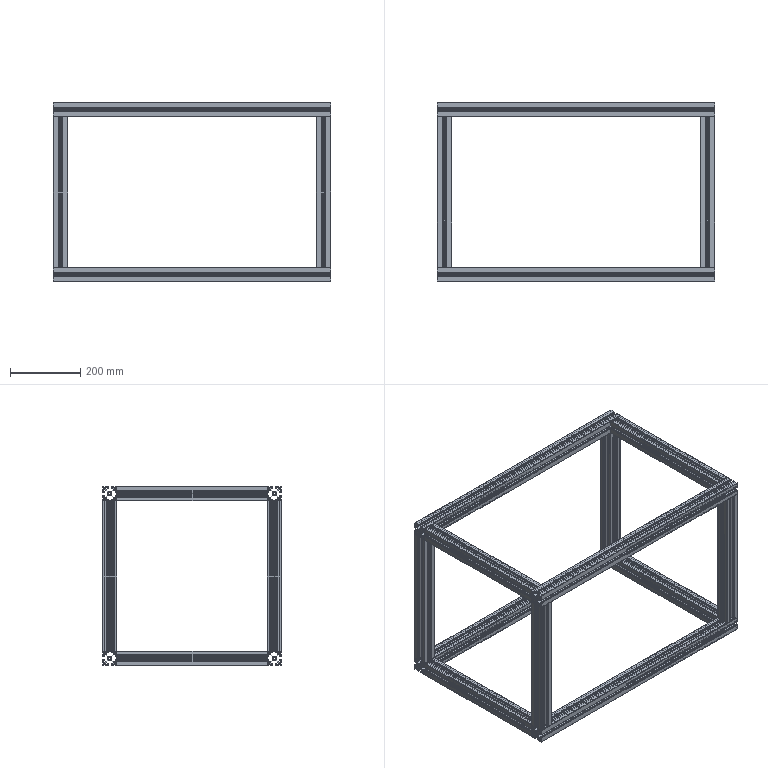Part | STEP file | Vibratory bowl feeder support frame_Default<machined> | 12 solids | 2076 faces | box 790 x 510 x 510 mm | volume 4425071 mm3 | cylinder 1092 | plane 984 | commonest cylinder face diameters 1 x528 0.6 x348 4 x96 4.9 x96 6.8 x24